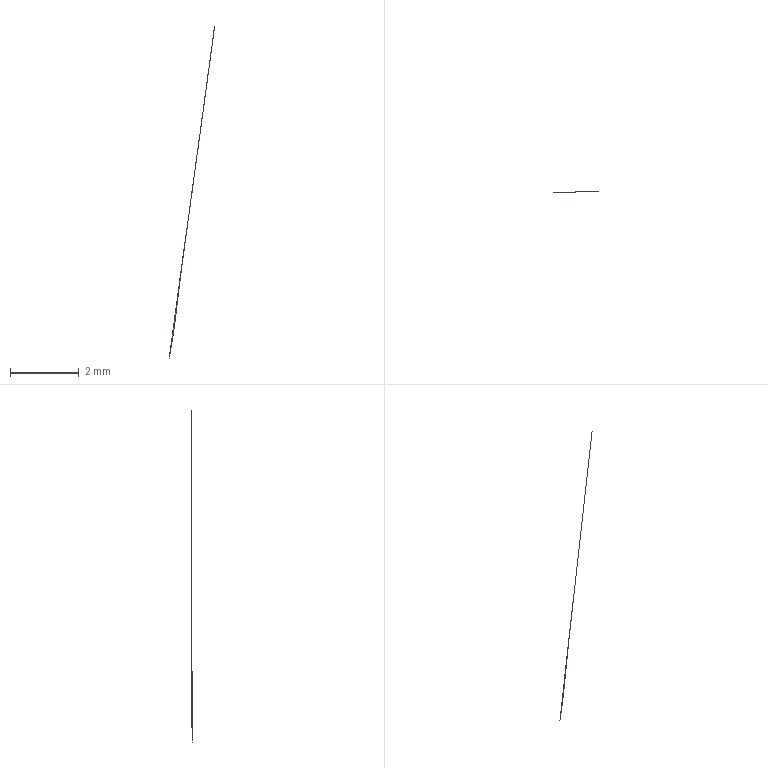Part | NX | features solid 2 | 1 solid | 2 faces | box 1.322 x 0.002198 x 9.66 mm | volume 0.0000237 mm3 | spline 2